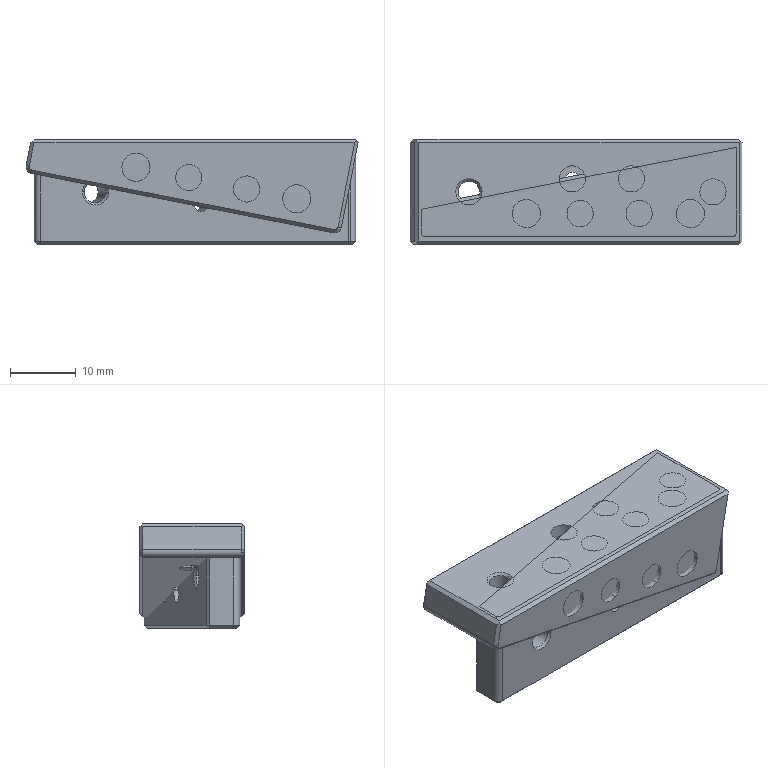Part | 2 solids | 118 faces | box 50.629 x 16.001 x 16.002 mm | volume 13679 mm3 | cylinder 46 | plane 40 | cone 24 | spline 8 | commonest cylinder face diameters 4 x16 2 x14 3.3 x8 4.3 x8